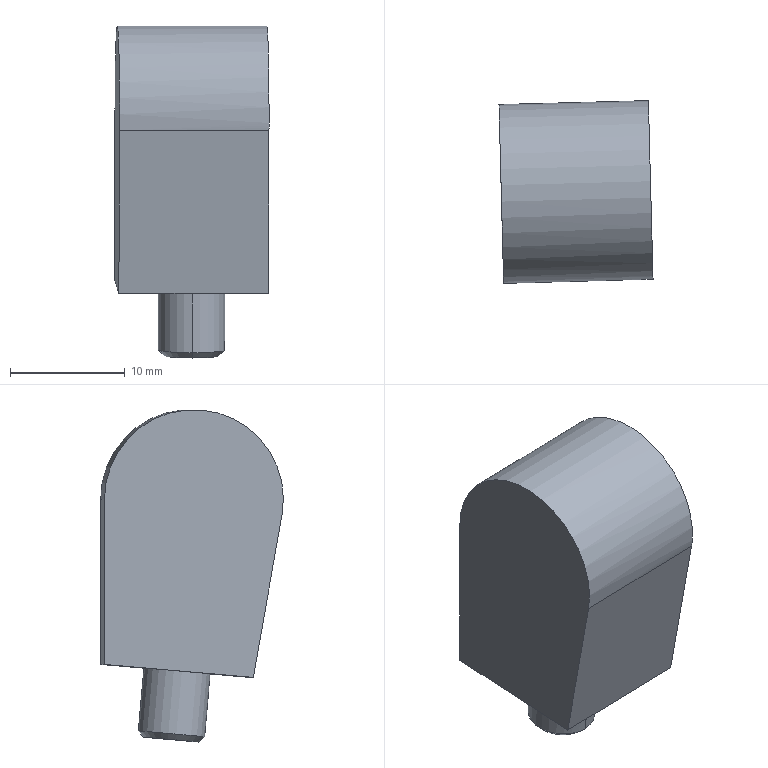Part | STEP file | 1_id1058_x_t | 1 solid | 11 faces | box 13.4 x 15.898 x 28.911 mm | volume 4184 mm3 | plane 6 | cylinder 3 | cone 2 | commonest cylinder face diameters 5.795 x2 15.565 x1
STEP:
#1=CARTESIAN_POINT('',(0.,0.,0.));
#2=DIRECTION('',(0.,0.,1.));
#3=DIRECTION('',(1.,0.,0.));
#4=AXIS2_PLACEMENT_3D('',#1,#2,#3);
#5=CARTESIAN_POINT('',(972.745,345.028,-29.863));
#6=VERTEX_POINT('',#5);
#7=CARTESIAN_POINT('',(972.733,345.49,-29.313));
#8=VERTEX_POINT('',#7);
#9=CARTESIAN_POINT('',(972.745,345.028,-29.863));
#10=DIRECTION('',(-0.01672,0.6426,0.766));
#11=VECTOR('',#10,1.);
#12=LINE('',#9,#11);
#13=CARTESIAN_POINT('',(972.807,342.627,-29.819));
#14=DIRECTION('',(0.002266,-0.08713,0.9962));
#15=DIRECTION('',(-0.02591,0.9959,0.08716));
#16=AXIS2_PLACEMENT_3D('',#13,#14,#15);
#17=CONICAL_SURFACE('',#16,2.644,0.7854);
#18=CARTESIAN_POINT('',(6.283,-0.254));
#19=DIRECTION('',(0.,1.));
#20=VECTOR('',#19,1.);
#21=LINE('',#18,#20);
#22=(GEOMETRIC_REPRESENTATION_CONTEXT(2)PARAMETRIC_REPRESENTATION_CONTEXT()REPRESENTATION_CONTEXT('',''));
#23=DEFINITIONAL_REPRESENTATION('',(#21),#22);
#24=PCURVE('',#17,#23);
#25=CARTESIAN_POINT('',(972.807,342.627,-29.819));
#26=DIRECTION('',(0.002266,-0.08713,0.9962));
#27=DIRECTION('',(-0.02591,0.9959,0.08716));
#28=AXIS2_PLACEMENT_3D('',#25,#26,#27);
#29=CONICAL_SURFACE('',#28,2.644,0.7854);
#30=CARTESIAN_POINT('',(0.,-0.254));
#31=DIRECTION('',(0.,1.));
#32=VECTOR('',#31,1.);
#33=LINE('',#30,#32);
#34=(GEOMETRIC_REPRESENTATION_CONTEXT(2)PARAMETRIC_REPRESENTATION_CONTEXT()REPRESENTATION_CONTEXT('',''));
#35=DEFINITIONAL_REPRESENTATION('',(#33),#34);
#36=PCURVE('',#29,#35);
#37=SURFACE_CURVE('',#12,(#24,#36),.PCURVE_S1.);
#38=EDGE_CURVE('',#6,#8,#37,.T.);
#39=ORIENTED_EDGE('',*,*,#38,.T.);
#40=CARTESIAN_POINT('',(972.883,339.719,-29.818));
#41=VERTEX_POINT('',#40);
#42=CARTESIAN_POINT('',(972.808,342.604,-29.565));
#43=DIRECTION('',(0.002266,-0.08713,0.9962));
#44=DIRECTION('',(0.02591,-0.9959,-0.08716));
#45=AXIS2_PLACEMENT_3D('',#42,#43,#44);
#46=CIRCLE('',#45,2.898);
#47=CARTESIAN_POINT('',(3.142,0.254));
#48=DIRECTION('',(1.,0.));
#49=VECTOR('',#48,1.);
#50=LINE('',#47,#49);
#51=(GEOMETRIC_REPRESENTATION_CONTEXT(2)PARAMETRIC_REPRESENTATION_CONTEXT()REPRESENTATION_CONTEXT('',''));
#52=DEFINITIONAL_REPRESENTATION('',(#50),#51);
#53=PCURVE('',#17,#52);
#54=CARTESIAN_POINT('',(972.82,342.126,-24.094));
#55=DIRECTION('',(-0.002266,0.08713,-0.9962));
#56=DIRECTION('',(-0.02591,0.9959,0.08716));
#57=AXIS2_PLACEMENT_3D('',#54,#55,#56);
#58=CYLINDRICAL_SURFACE('',#57,2.898);
#59=CARTESIAN_POINT('',(3.142,5.492));
#60=DIRECTION('',(-1.,0.));
#61=VECTOR('',#60,1.);
#62=LINE('',#59,#61);
#63=(GEOMETRIC_REPRESENTATION_CONTEXT(2)PARAMETRIC_REPRESENTATION_CONTEXT()REPRESENTATION_CONTEXT('',''));
#64=DEFINITIONAL_REPRESENTATION('',(#62),#63);
#65=PCURVE('',#58,#64);
#66=SURFACE_CURVE('',#46,(#53,#65),.PCURVE_S1.);
#67=EDGE_CURVE('',#41,#8,#66,.T.);
#68=ORIENTED_EDGE('',*,*,#67,.F.);
#69=CARTESIAN_POINT('',(972.869,340.269,-30.28));
#70=VERTEX_POINT('',#69);
#71=CARTESIAN_POINT('',(972.869,340.269,-30.28));
#72=DIRECTION('',(-0.01992,0.7658,-0.6428));
#73=VECTOR('',#72,1.);
#74=LINE('',#71,#73);
#75=CARTESIAN_POINT('',(3.142,-0.254));
#76=DIRECTION('',(0.,-1.));
#77=VECTOR('',#76,1.);
#78=LINE('',#75,#77);
#79=(GEOMETRIC_REPRESENTATION_CONTEXT(2)PARAMETRIC_REPRESENTATION_CONTEXT()REPRESENTATION_CONTEXT('',''));
#80=DEFINITIONAL_REPRESENTATION('',(#78),#79);
#81=PCURVE('',#17,#80);
#82=CARTESIAN_POINT('',(3.142,-0.254));
#83=DIRECTION('',(0.,-1.));
#84=VECTOR('',#83,1.);
#85=LINE('',#82,#84);
#86=(GEOMETRIC_REPRESENTATION_CONTEXT(2)PARAMETRIC_REPRESENTATION_CONTEXT()REPRESENTATION_CONTEXT('',''));
#87=DEFINITIONAL_REPRESENTATION('',(#85),#86);
#88=PCURVE('',#29,#87);
#89=SURFACE_CURVE('',#74,(#81,#88),.PCURVE_S1.);
#90=EDGE_CURVE('',#41,#70,#89,.T.);
#91=ORIENTED_EDGE('',*,*,#90,.T.);
#92=CARTESIAN_POINT('',(972.807,342.649,-30.072));
#93=DIRECTION('',(-0.002266,0.08713,-0.9962));
#94=DIRECTION('',(-0.02591,0.9959,0.08716));
#95=AXIS2_PLACEMENT_3D('',#92,#93,#94);
#96=CIRCLE('',#95,2.39);
#97=CARTESIAN_POINT('',(6.283,-0.254));
#98=DIRECTION('',(-1.,0.));
#99=VECTOR('',#98,1.);
#100=LINE('',#97,#99);
#101=(GEOMETRIC_REPRESENTATION_CONTEXT(2)PARAMETRIC_REPRESENTATION_CONTEXT()REPRESENTATION_CONTEXT('',''));
#102=DEFINITIONAL_REPRESENTATION('',(#100),#101);
#103=PCURVE('',#17,#102);
#104=CARTESIAN_POINT('',(972.807,342.649,-30.072));
#105=DIRECTION('',(-0.002266,0.08713,-0.9962));
#106=DIRECTION('',(0.8426,0.5366,0.04501));
#107=AXIS2_PLACEMENT_3D('',#104,#105,#106);
#108=PLANE('',#107);
#109=CARTESIAN_POINT('',(0.,0.));
#110=DIRECTION('',(0.5165,-0.8563));
#111=AXIS2_PLACEMENT_2D('',#109,#110);
#112=CIRCLE('',#111,2.39);
#113=(GEOMETRIC_REPRESENTATION_CONTEXT(2)PARAMETRIC_REPRESENTATION_CONTEXT()REPRESENTATION_CONTEXT('',''));
#114=DEFINITIONAL_REPRESENTATION('',(#112),#113);
#115=PCURVE('',#108,#114);
#116=SURFACE_CURVE('',#96,(#103,#115),.PCURVE_S1.);
#117=EDGE_CURVE('',#6,#70,#116,.T.);
#118=ORIENTED_EDGE('',*,*,#117,.F.);
#119=EDGE_LOOP('',(#39,#68,#91,#118));
#120=FACE_BOUND('',#119,.T.);
#121=ADVANCED_FACE('',(#120),#17,.T.);
#122=CARTESIAN_POINT('',(972.807,342.649,-30.072));
#123=DIRECTION('',(-0.002266,0.08713,-0.9962));
#124=DIRECTION('',(0.02591,-0.9959,-0.08716));
#125=AXIS2_PLACEMENT_3D('',#122,#123,#124);
#126=CIRCLE('',#125,2.39);
#127=CARTESIAN_POINT('',(0.,0.));
#128=DIRECTION('',(-0.5165,0.8563));
#129=AXIS2_PLACEMENT_2D('',#127,#128);
#130=CIRCLE('',#129,2.39);
#131=(GEOMETRIC_REPRESENTATION_CONTEXT(2)PARAMETRIC_REPRESENTATION_CONTEXT()REPRESENTATION_CONTEXT('',''));
#132=DEFINITIONAL_REPRESENTATION('',(#130),#131);
#133=PCURVE('',#108,#132);
#134=CARTESIAN_POINT('',(3.142,-0.254));
#135=DIRECTION('',(-1.,0.));
#136=VECTOR('',#135,1.);
#137=LINE('',#134,#136);
#138=(GEOMETRIC_REPRESENTATION_CONTEXT(2)PARAMETRIC_REPRESENTATION_CONTEXT()REPRESENTATION_CONTEXT('',''));
#139=DEFINITIONAL_REPRESENTATION('',(#137),#138);
#140=PCURVE('',#29,#139);
#141=SURFACE_CURVE('',#126,(#133,#140),.PCURVE_S1.);
#142=EDGE_CURVE('',#70,#6,#141,.T.);
#143=ORIENTED_EDGE('',*,*,#142,.T.);
#144=ORIENTED_EDGE('',*,*,#117,.T.);
#145=EDGE_LOOP('',(#143,#144));
#146=FACE_BOUND('',#145,.T.);
#147=ADVANCED_FACE('',(#146),#108,.T.);
#148=ORIENTED_EDGE('',*,*,#90,.F.);
#149=CARTESIAN_POINT('',(972.808,342.604,-29.565));
#150=DIRECTION('',(0.002266,-0.08713,0.9962));
#151=DIRECTION('',(-0.02591,0.9959,0.08716));
#152=AXIS2_PLACEMENT_3D('',#149,#150,#151);
#153=CIRCLE('',#152,2.898);
#154=CARTESIAN_POINT('',(0.,0.254));
#155=DIRECTION('',(1.,0.));
#156=VECTOR('',#155,1.);
#157=LINE('',#154,#156);
#158=(GEOMETRIC_REPRESENTATION_CONTEXT(2)PARAMETRIC_REPRESENTATION_CONTEXT()REPRESENTATION_CONTEXT('',''));
#159=DEFINITIONAL_REPRESENTATION('',(#157),#158);
#160=PCURVE('',#29,#159);
#161=CARTESIAN_POINT('',(972.82,342.126,-24.094));
#162=DIRECTION('',(-0.002266,0.08713,-0.9962));
#163=DIRECTION('',(-0.02591,0.9959,0.08716));
#164=AXIS2_PLACEMENT_3D('',#161,#162,#163);
#165=CYLINDRICAL_SURFACE('',#164,2.898);
#166=CARTESIAN_POINT('',(6.283,5.492));
#167=DIRECTION('',(-1.,0.));
#168=VECTOR('',#167,1.);
#169=LINE('',#166,#168);
#170=(GEOMETRIC_REPRESENTATION_CONTEXT(2)PARAMETRIC_REPRESENTATION_CONTEXT()REPRESENTATION_CONTEXT('',''));
#171=DEFINITIONAL_REPRESENTATION('',(#169),#170);
#172=PCURVE('',#165,#171);
#173=SURFACE_CURVE('',#153,(#160,#172),.PCURVE_S1.);
#174=EDGE_CURVE('',#8,#41,#173,.T.);
#175=ORIENTED_EDGE('',*,*,#174,.F.);
#176=ORIENTED_EDGE('',*,*,#38,.F.);
#177=ORIENTED_EDGE('',*,*,#142,.F.);
#178=EDGE_LOOP('',(#148,#175,#176,#177));
#179=FACE_BOUND('',#178,.T.);
#180=ADVANCED_FACE('',(#179),#29,.T.);
#181=CARTESIAN_POINT('',(972.895,339.24,-24.347));
#182=VERTEX_POINT('',#181);
#183=CARTESIAN_POINT('',(972.895,339.24,-24.347));
#184=DIRECTION('',(0.002266,-0.08713,0.9962));
#185=VECTOR('',#184,1.);
#186=LINE('',#183,#185);
#187=CARTESIAN_POINT('',(3.142,0.));
#188=DIRECTION('',(0.,-1.));
#189=VECTOR('',#188,1.);
#190=LINE('',#187,#189);
#191=(GEOMETRIC_REPRESENTATION_CONTEXT(2)PARAMETRIC_REPRESENTATION_CONTEXT()REPRESENTATION_CONTEXT('',''));
#192=DEFINITIONAL_REPRESENTATION('',(#190),#191);
#193=PCURVE('',#165,#192);
#194=CARTESIAN_POINT('',(3.142,0.));
#195=DIRECTION('',(0.,-1.));
#196=VECTOR('',#195,1.);
#197=LINE('',#194,#196);
#198=(GEOMETRIC_REPRESENTATION_CONTEXT(2)PARAMETRIC_REPRESENTATION_CONTEXT()REPRESENTATION_CONTEXT('',''));
#199=DEFINITIONAL_REPRESENTATION('',(#197),#198);
#200=PCURVE('',#58,#199);
#201=SURFACE_CURVE('',#186,(#193,#200),.PCURVE_S1.);
#202=EDGE_CURVE('',#41,#182,#201,.T.);
#203=ORIENTED_EDGE('',*,*,#202,.T.);
#204=CARTESIAN_POINT('',(972.745,345.011,-23.842));
#205=VERTEX_POINT('',#204);
#206=CARTESIAN_POINT('',(972.82,342.126,-24.094));
#207=DIRECTION('',(0.002266,-0.08713,0.9962));
#208=DIRECTION('',(-0.02591,0.9959,0.08716));
#209=AXIS2_PLACEMENT_3D('',#206,#207,#208);
#210=CIRCLE('',#209,2.898);
#211=CARTESIAN_POINT('',(6.283,0.));
#212=DIRECTION('',(-1.,0.));
#213=VECTOR('',#212,1.);
#214=LINE('',#211,#213);
#215=(GEOMETRIC_REPRESENTATION_CONTEXT(2)PARAMETRIC_REPRESENTATION_CONTEXT()REPRESENTATION_CONTEXT('',''));
#216=DEFINITIONAL_REPRESENTATION('',(#214),#215);
#217=PCURVE('',#165,#216);
#218=CARTESIAN_POINT('',(979.15,348.768,-23.528));
#219=DIRECTION('',(-0.002266,0.08713,-0.9962));
#220=DIRECTION('',(0.8426,0.5366,0.04501));
#221=AXIS2_PLACEMENT_3D('',#218,#219,#220);
#222=PLANE('',#221);
#223=CARTESIAN_POINT('',(-7.427,-0.2723));
#224=CARTESIAN_POINT('',(-11.724,-2.864));
#225=CARTESIAN_POINT('',(-11.82,2.153));
#226=CARTESIAN_POINT('',(-11.916,7.171));
#227=CARTESIAN_POINT('',(-7.523,4.745));
#228=CARTESIAN_POINT('',(-3.129,2.32));
#229=CARTESIAN_POINT('',(-7.427,-0.2723));
#230=(BOUNDED_CURVE()B_SPLINE_CURVE(2,(#223,#224,#225,#226,#227,#228,#229),.UNSPECIFIED.,.T.,.F.)B_SPLINE_CURVE_WITH_KNOTS((1,2,2,2,2,1),(-2.094,0.,2.094,4.189,6.283,8.378),.UNSPECIFIED.)CURVE()GEOMETRIC_REPRESENTATION_ITEM()RATIONAL_B_SPLINE_CURVE((1.,0.5,1.,0.5,1.,0.5,1.))REPRESENTATION_ITEM(''));
#231=(GEOMETRIC_REPRESENTATION_CONTEXT(2)PARAMETRIC_REPRESENTATION_CONTEXT()REPRESENTATION_CONTEXT('',''));
#232=DEFINITIONAL_REPRESENTATION('',(#230),#231);
#233=PCURVE('',#222,#232);
#234=SURFACE_CURVE('',#210,(#217,#233),.PCURVE_S1.);
#235=EDGE_CURVE('',#205,#182,#234,.T.);
#236=ORIENTED_EDGE('',*,*,#235,.F.);
#237=CARTESIAN_POINT('',(972.745,345.011,-23.842));
#238=DIRECTION('',(-0.002266,0.08713,-0.9962));
#239=VECTOR('',#238,1.);
#240=LINE('',#237,#239);
#241=CARTESIAN_POINT('',(6.283,0.));
#242=DIRECTION('',(0.,1.));
#243=VECTOR('',#242,1.);
#244=LINE('',#241,#243);
#245=(GEOMETRIC_REPRESENTATION_CONTEXT(2)PARAMETRIC_REPRESENTATION_CONTEXT()REPRESENTATION_CONTEXT('',''));
#246=DEFINITIONAL_REPRESENTATION('',(#244),#245);
#247=PCURVE('',#165,#246);
#248=CARTESIAN_POINT('',(0.,0.));
#249=DIRECTION('',(0.,1.));
#250=VECTOR('',#249,1.);
#251=LINE('',#248,#250);
#252=(GEOMETRIC_REPRESENTATION_CONTEXT(2)PARAMETRIC_REPRESENTATION_CONTEXT()REPRESENTATION_CONTEXT('',''));
#253=DEFINITIONAL_REPRESENTATION('',(#251),#252);
#254=PCURVE('',#58,#253);
#255=SURFACE_CURVE('',#240,(#247,#254),.PCURVE_S1.);
#256=EDGE_CURVE('',#205,#8,#255,.T.);
#257=ORIENTED_EDGE('',*,*,#256,.T.);
#258=ORIENTED_EDGE('',*,*,#174,.T.);
#259=EDGE_LOOP('',(#203,#236,#257,#258));
#260=FACE_BOUND('',#259,.T.);
#261=ADVANCED_FACE('',(#260),#165,.T.);
#262=ORIENTED_EDGE('',*,*,#256,.F.);
#263=CARTESIAN_POINT('',(972.82,342.126,-24.094));
#264=DIRECTION('',(0.002266,-0.08713,0.9962));
#265=DIRECTION('',(0.02591,-0.9959,-0.08716));
#266=AXIS2_PLACEMENT_3D('',#263,#264,#265);
#267=CIRCLE('',#266,2.898);
#268=CARTESIAN_POINT('',(3.142,0.));
#269=DIRECTION('',(-1.,0.));
#270=VECTOR('',#269,1.);
#271=LINE('',#268,#270);
#272=(GEOMETRIC_REPRESENTATION_CONTEXT(2)PARAMETRIC_REPRESENTATION_CONTEXT()REPRESENTATION_CONTEXT('',''));
#273=DEFINITIONAL_REPRESENTATION('',(#271),#272);
#274=PCURVE('',#58,#273);
#275=CARTESIAN_POINT('',(-10.42,4.69));
#276=CARTESIAN_POINT('',(-6.122,7.282));
#277=CARTESIAN_POINT('',(-6.026,2.264));
#278=CARTESIAN_POINT('',(-5.93,-2.753));
#279=CARTESIAN_POINT('',(-10.324,-0.3278));
#280=CARTESIAN_POINT('',(-14.717,2.098));
#281=CARTESIAN_POINT('',(-10.42,4.69));
#282=(BOUNDED_CURVE()B_SPLINE_CURVE(2,(#275,#276,#277,#278,#279,#280,#281),.UNSPECIFIED.,.T.,.F.)B_SPLINE_CURVE_WITH_KNOTS((1,2,2,2,2,1),(-2.094,0.,2.094,4.189,6.283,8.378),.UNSPECIFIED.)CURVE()GEOMETRIC_REPRESENTATION_ITEM()RATIONAL_B_SPLINE_CURVE((1.,0.5,1.,0.5,1.,0.5,1.))REPRESENTATION_ITEM(''));
#283=(GEOMETRIC_REPRESENTATION_CONTEXT(2)PARAMETRIC_REPRESENTATION_CONTEXT()REPRESENTATION_CONTEXT('',''));
#284=DEFINITIONAL_REPRESENTATION('',(#282),#283);
#285=PCURVE('',#222,#284);
#286=SURFACE_CURVE('',#267,(#274,#285),.PCURVE_S1.);
#287=EDGE_CURVE('',#182,#205,#286,.T.);
#288=ORIENTED_EDGE('',*,*,#287,.F.);
#289=ORIENTED_EDGE('',*,*,#202,.F.);
#290=ORIENTED_EDGE('',*,*,#67,.T.);
#291=EDGE_LOOP('',(#262,#288,#289,#290));
#292=FACE_BOUND('',#291,.T.);
#293=ADVANCED_FACE('',(#292),#58,.T.);
#294=CARTESIAN_POINT('',(966.154,348.43,-23.528));
#295=VERTEX_POINT('',#294);
#296=CARTESIAN_POINT('',(979.15,348.768,-23.528));
#297=VERTEX_POINT('',#296);
#298=CARTESIAN_POINT('',(966.154,348.43,-23.528));
#299=DIRECTION('',(0.9997,0.02601,0.));
#300=VECTOR('',#299,1.);
#301=LINE('',#298,#300);
#302=CARTESIAN_POINT('',(-11.132,-6.714));
#303=DIRECTION('',(0.8563,0.5165));
#304=VECTOR('',#303,1.);
#305=LINE('',#302,#304);
#306=(GEOMETRIC_REPRESENTATION_CONTEXT(2)PARAMETRIC_REPRESENTATION_CONTEXT()REPRESENTATION_CONTEXT('',''));
#307=DEFINITIONAL_REPRESENTATION('',(#305),#306);
#308=PCURVE('',#222,#307);
#309=CARTESIAN_POINT('',(979.15,348.768,-9.151));
#310=DIRECTION('',(-0.02601,0.9997,0.));
#311=DIRECTION('',(0.,0.,-1.));
#312=AXIS2_PLACEMENT_3D('',#309,#310,#311);
#313=PLANE('',#312);
#314=CARTESIAN_POINT('',(14.376,13.));
#315=DIRECTION('',(0.,-1.));
#316=VECTOR('',#315,1.);
#317=LINE('',#314,#316);
#318=(GEOMETRIC_REPRESENTATION_CONTEXT(2)PARAMETRIC_REPRESENTATION_CONTEXT()REPRESENTATION_CONTEXT('',''));
#319=DEFINITIONAL_REPRESENTATION('',(#317),#318);
#320=PCURVE('',#313,#319);
#321=SURFACE_CURVE('',#301,(#308,#320),.PCURVE_S1.);
#322=EDGE_CURVE('',#295,#297,#321,.T.);
#323=ORIENTED_EDGE('',*,*,#322,.T.);
#324=CARTESIAN_POINT('',(979.487,335.822,-24.661));
#325=VERTEX_POINT('',#324);
#326=CARTESIAN_POINT('',(979.487,335.822,-24.661));
#327=DIRECTION('',(-0.02591,0.9959,0.08716));
#328=VECTOR('',#327,1.);
#329=LINE('',#326,#328);
#330=CARTESIAN_POINT('',(-6.714,11.132));
#331=DIRECTION('',(0.5165,-0.8563));
#332=VECTOR('',#331,1.);
#333=LINE('',#330,#332);
#334=(GEOMETRIC_REPRESENTATION_CONTEXT(2)PARAMETRIC_REPRESENTATION_CONTEXT()REPRESENTATION_CONTEXT('',''));
#335=DEFINITIONAL_REPRESENTATION('',(#333),#334);
#336=PCURVE('',#222,#335);
#337=CARTESIAN_POINT('',(979.352,340.988,-9.151));
#338=DIRECTION('',(0.9997,0.02601,0.));
#339=DIRECTION('',(0.02601,-0.9997,0.));
#340=AXIS2_PLACEMENT_3D('',#337,#338,#339);
#341=PLANE('',#340);
#342=CARTESIAN_POINT('',(5.168,15.509));
#343=DIRECTION('',(-0.9962,-0.08716));
#344=VECTOR('',#343,1.);
#345=LINE('',#342,#344);
#346=(GEOMETRIC_REPRESENTATION_CONTEXT(2)PARAMETRIC_REPRESENTATION_CONTEXT()REPRESENTATION_CONTEXT('',''));
#347=DEFINITIONAL_REPRESENTATION('',(#345),#346);
#348=PCURVE('',#341,#347);
#349=SURFACE_CURVE('',#329,(#336,#348),.PCURVE_S1.);
#350=EDGE_CURVE('',#325,#297,#349,.T.);
#351=ORIENTED_EDGE('',*,*,#350,.F.);
#352=CARTESIAN_POINT('',(966.491,335.484,-24.661));
#353=VERTEX_POINT('',#352);
#354=CARTESIAN_POINT('',(966.491,335.484,-24.661));
#355=DIRECTION('',(0.9997,0.02601,0.));
#356=VECTOR('',#355,1.);
#357=LINE('',#354,#356);
#358=CARTESIAN_POINT('',(-17.846,4.418));
#359=DIRECTION('',(0.8563,0.5165));
#360=VECTOR('',#359,1.);
#361=LINE('',#358,#360);
#362=(GEOMETRIC_REPRESENTATION_CONTEXT(2)PARAMETRIC_REPRESENTATION_CONTEXT()REPRESENTATION_CONTEXT('',''));
#363=DEFINITIONAL_REPRESENTATION('',(#361),#362);
#364=PCURVE('',#222,#363);
#365=CARTESIAN_POINT('',(979.551,333.326,-10.503));
#366=DIRECTION('',(-0.02561,0.9845,0.1736));
#367=DIRECTION('',(0.2732,0.174,-0.9461));
#368=AXIS2_PLACEMENT_3D('',#365,#366,#367);
#369=PLANE('',#368);
#370=CARTESIAN_POINT('',(10.202,16.48));
#371=DIRECTION('',(0.2776,-0.9607));
#372=VECTOR('',#371,1.);
#373=LINE('',#370,#372);
#374=(GEOMETRIC_REPRESENTATION_CONTEXT(2)PARAMETRIC_REPRESENTATION_CONTEXT()REPRESENTATION_CONTEXT('',''));
#375=DEFINITIONAL_REPRESENTATION('',(#373),#374);
#376=PCURVE('',#369,#375);
#377=SURFACE_CURVE('',#357,(#364,#376),.PCURVE_S1.);
#378=EDGE_CURVE('',#353,#325,#377,.T.);
#379=ORIENTED_EDGE('',*,*,#378,.F.);
#380=CARTESIAN_POINT('',(966.491,335.484,-24.661));
#381=DIRECTION('',(-0.02591,0.9959,0.08716));
#382=VECTOR('',#381,1.);
#383=LINE('',#380,#382);
#384=CARTESIAN_POINT('',(-17.846,4.418));
#385=DIRECTION('',(0.5165,-0.8563));
#386=VECTOR('',#385,1.);
#387=LINE('',#384,#386);
#388=(GEOMETRIC_REPRESENTATION_CONTEXT(2)PARAMETRIC_REPRESENTATION_CONTEXT()REPRESENTATION_CONTEXT('',''));
#389=DEFINITIONAL_REPRESENTATION('',(#387),#388);
#390=PCURVE('',#222,#389);
#391=CARTESIAN_POINT('',(966.357,340.65,-9.151));
#392=DIRECTION('',(0.9997,0.02601,0.));
#393=DIRECTION('',(0.02601,-0.9997,0.));
#394=AXIS2_PLACEMENT_3D('',#391,#392,#393);
#395=PLANE('',#394);
#396=CARTESIAN_POINT('',(5.168,15.509));
#397=DIRECTION('',(-0.9962,-0.08716));
#398=VECTOR('',#397,1.);
#399=LINE('',#396,#398);
#400=(GEOMETRIC_REPRESENTATION_CONTEXT(2)PARAMETRIC_REPRESENTATION_CONTEXT()REPRESENTATION_CONTEXT('',''));
#401=DEFINITIONAL_REPRESENTATION('',(#399),#400);
#402=PCURVE('',#395,#401);
#403=SURFACE_CURVE('',#383,(#390,#402),.PCURVE_S1.);
#404=EDGE_CURVE('',#353,#295,#403,.T.);
#405=ORIENTED_EDGE('',*,*,#404,.T.);
#406=EDGE_LOOP('',(#323,#351,#379,#405));
#407=FACE_BOUND('',#406,.T.);
#408=ORIENTED_EDGE('',*,*,#287,.T.);
#409=ORIENTED_EDGE('',*,*,#235,.T.);
#410=EDGE_LOOP('',(#408,#409));
#411=FACE_BOUND('',#410,.T.);
#412=ADVANCED_FACE('',(#407,#411),#222,.T.);
#413=CARTESIAN_POINT('',(966.556,332.988,-10.503));
#414=VERTEX_POINT('',#413);
#415=CARTESIAN_POINT('',(966.491,335.484,-24.661));
#416=DIRECTION('',(0.004516,-0.1736,0.9848));
#417=VECTOR('',#416,1.);
#418=LINE('',#415,#417);
#419=CARTESIAN_POINT('',(5.168,15.509));
#420=DIRECTION('',(0.1736,-0.9848));
#421=VECTOR('',#420,1.);
#422=LINE('',#419,#421);
#423=(GEOMETRIC_REPRESENTATION_CONTEXT(2)PARAMETRIC_REPRESENTATION_CONTEXT()REPRESENTATION_CONTEXT('',''));
#424=DEFINITIONAL_REPRESENTATION('',(#422),#423);
#425=PCURVE('',#395,#424);
#426=CARTESIAN_POINT('',(10.202,16.48));
#427=DIRECTION('',(-0.9607,-0.2776));
#428=VECTOR('',#427,1.);
#429=LINE('',#426,#428);
#430=(GEOMETRIC_REPRESENTATION_CONTEXT(2)PARAMETRIC_REPRESENTATION_CONTEXT()REPRESENTATION_CONTEXT('',''));
#431=DEFINITIONAL_REPRESENTATION('',(#429),#430);
#432=PCURVE('',#369,#431);
#433=SURFACE_CURVE('',#418,(#425,#432),.PCURVE_S1.);
#434=EDGE_CURVE('',#353,#414,#433,.T.);
#435=ORIENTED_EDGE('',*,*,#434,.T.);
#436=CARTESIAN_POINT('',(966.374,339.972,-1.398));
#437=VERTEX_POINT('',#436);
#438=CARTESIAN_POINT('',(966.357,340.65,-9.151));
#439=DIRECTION('',(-0.9997,-0.02601,0.));
#440=DIRECTION('',(0.02561,-0.9845,-0.1736));
#441=AXIS2_PLACEMENT_3D('',#438,#439,#440);
#442=CIRCLE('',#441,7.783);
#443=CARTESIAN_POINT('',(7.664,1.351));
#444=CARTESIAN_POINT('',(10.005,-11.924));
#445=CARTESIAN_POINT('',(-2.662,-7.313));
#446=CARTESIAN_POINT('',(-15.329,-2.703));
#447=CARTESIAN_POINT('',(-5.003,5.962));
#448=CARTESIAN_POINT('',(5.324,14.627));
#449=CARTESIAN_POINT('',(7.664,1.351));
#450=(BOUNDED_CURVE()B_SPLINE_CURVE(2,(#443,#444,#445,#446,#447,#448,#449),.UNSPECIFIED.,.T.,.F.)B_SPLINE_CURVE_WITH_KNOTS((1,2,2,2,2,1),(-2.094,0.,2.094,4.189,6.283,8.378),.UNSPECIFIED.)CURVE()GEOMETRIC_REPRESENTATION_ITEM()RATIONAL_B_SPLINE_CURVE((1.,0.5,1.,0.5,1.,0.5,1.))REPRESENTATION_ITEM(''));
#451=(GEOMETRIC_REPRESENTATION_CONTEXT(2)PARAMETRIC_REPRESENTATION_CONTEXT()REPRESENTATION_CONTEXT('',''));
#452=DEFINITIONAL_REPRESENTATION('',(#450),#451);
#453=PCURVE('',#395,#452);
#454=CARTESIAN_POINT('',(979.352,340.988,-9.151));
#455=DIRECTION('',(-0.9997,-0.02601,0.));
#456=DIRECTION('',(-0.002266,0.08713,-0.9962));
#457=AXIS2_PLACEMENT_3D('',#454,#455,#456);
#458=CYLINDRICAL_SURFACE('',#457,7.783);
#459=CARTESIAN_POINT('',(1.484,13.));
#460=DIRECTION('',(1.,0.));
#461=VECTOR('',#460,1.);
#462=LINE('',#459,#461);
#463=(GEOMETRIC_REPRESENTATION_CONTEXT(2)PARAMETRIC_REPRESENTATION_CONTEXT()REPRESENTATION_CONTEXT('',''));
#464=DEFINITIONAL_REPRESENTATION('',(#462),#463);
#465=PCURVE('',#458,#464);
#466=SURFACE_CURVE('',#442,(#453,#465),.PCURVE_S1.);
#467=EDGE_CURVE('',#414,#437,#466,.T.);
#468=ORIENTED_EDGE('',*,*,#467,.T.);
#469=CARTESIAN_POINT('',(966.154,348.43,-9.151));
#470=VERTEX_POINT('',#469);
#471=CARTESIAN_POINT('',(966.357,340.65,-9.151));
#472=DIRECTION('',(-0.9997,-0.02601,0.));
#473=DIRECTION('',(0.002266,-0.08713,0.9962));
#474=AXIS2_PLACEMENT_3D('',#471,#472,#473);
#475=CIRCLE('',#474,7.783);
#476=CARTESIAN_POINT('',(0.6783,-7.753));
#477=CARTESIAN_POINT('',(-12.75,-8.928));
#478=CARTESIAN_POINT('',(-7.053,3.289));
#479=CARTESIAN_POINT('',(-1.357,15.506));
#480=CARTESIAN_POINT('',(6.375,4.464));
#481=CARTESIAN_POINT('',(14.107,-6.578));
#482=CARTESIAN_POINT('',(0.6783,-7.753));
#483=(BOUNDED_CURVE()B_SPLINE_CURVE(2,(#476,#477,#478,#479,#480,#481,#482),.UNSPECIFIED.,.T.,.F.)B_SPLINE_CURVE_WITH_KNOTS((1,2,2,2,2,1),(-2.094,0.,2.094,4.189,6.283,8.378),.UNSPECIFIED.)CURVE()GEOMETRIC_REPRESENTATION_ITEM()RATIONAL_B_SPLINE_CURVE((1.,0.5,1.,0.5,1.,0.5,1.))REPRESENTATION_ITEM(''));
#484=(GEOMETRIC_REPRESENTATION_CONTEXT(2)PARAMETRIC_REPRESENTATION_CONTEXT()REPRESENTATION_CONTEXT('',''));
#485=DEFINITIONAL_REPRESENTATION('',(#483),#484);
#486=PCURVE('',#395,#485);
#487=CARTESIAN_POINT('',(3.142,13.));
#488=DIRECTION('',(1.,0.));
#489=VECTOR('',#488,1.);
#490=LINE('',#487,#489);
#491=(GEOMETRIC_REPRESENTATION_CONTEXT(2)PARAMETRIC_REPRESENTATION_CONTEXT()REPRESENTATION_CONTEXT('',''));
#492=DEFINITIONAL_REPRESENTATION('',(#490),#491);
#493=PCURVE('',#458,#492);
#494=SURFACE_CURVE('',#475,(#486,#493),.PCURVE_S1.);
#495=EDGE_CURVE('',#437,#470,#494,.T.);
#496=ORIENTED_EDGE('',*,*,#495,.T.);
#497=CARTESIAN_POINT('',(966.154,348.43,-23.528));
#498=DIRECTION('',(0.,0.,1.));
#499=VECTOR('',#498,1.);
#500=LINE('',#497,#499);
#501=CARTESIAN_POINT('',(-7.783,14.376));
#502=DIRECTION('',(0.,-1.));
#503=VECTOR('',#502,1.);
#504=LINE('',#501,#503);
#505=(GEOMETRIC_REPRESENTATION_CONTEXT(2)PARAMETRIC_REPRESENTATION_CONTEXT()REPRESENTATION_CONTEXT('',''));
#506=DEFINITIONAL_REPRESENTATION('',(#504),#505);
#507=PCURVE('',#395,#506);
#508=CARTESIAN_POINT('',(14.376,13.));
#509=DIRECTION('',(-1.,0.));
#510=VECTOR('',#509,1.);
#511=LINE('',#508,#510);
#512=(GEOMETRIC_REPRESENTATION_CONTEXT(2)PARAMETRIC_REPRESENTATION_CONTEXT()REPRESENTATION_CONTEXT('',''));
#513=DEFINITIONAL_REPRESENTATION('',(#511),#512);
#514=PCURVE('',#313,#513);
#515=SURFACE_CURVE('',#500,(#507,#514),.PCURVE_S1.);
#516=EDGE_CURVE('',#295,#470,#515,.T.);
#517=ORIENTED_EDGE('',*,*,#516,.F.);
#518=ORIENTED_EDGE('',*,*,#404,.F.);
#519=EDGE_LOOP('',(#435,#468,#496,#517,#518));
#520=FACE_BOUND('',#519,.T.);
#521=ADVANCED_FACE('',(#520),#395,.F.);
#522=CARTESIAN_POINT('',(979.15,348.768,-9.151));
#523=VERTEX_POINT('',#522);
#524=CARTESIAN_POINT('',(979.15,348.768,-9.151));
#525=DIRECTION('',(-0.9997,-0.02601,0.));
#526=VECTOR('',#525,1.);
#527=LINE('',#524,#526);
#528=CARTESIAN_POINT('',(0.,0.));
#529=DIRECTION('',(0.,1.));
#530=VECTOR('',#529,1.);
#531=LINE('',#528,#530);
#532=(GEOMETRIC_REPRESENTATION_CONTEXT(2)PARAMETRIC_REPRESENTATION_CONTEXT()REPRESENTATION_CONTEXT('',''));
#533=DEFINITIONAL_REPRESENTATION('',(#531),#532);
#534=PCURVE('',#313,#533);
#535=CARTESIAN_POINT('',(4.8,0.));
#536=DIRECTION('',(0.,1.));
#537=VECTOR('',#536,1.);
#538=LINE('',#535,#537);
#539=(GEOMETRIC_REPRESENTATION_CONTEXT(2)PARAMETRIC_REPRESENTATION_CONTEXT()REPRESENTATION_CONTEXT('',''));
#540=DEFINITIONAL_REPRESENTATION('',(#538),#539);
#541=PCURVE('',#458,#540);
#542=SURFACE_CURVE('',#527,(#534,#541),.PCURVE_S1.);
#543=EDGE_CURVE('',#523,#470,#542,.T.);
#544=ORIENTED_EDGE('',*,*,#543,.F.);
#545=CARTESIAN_POINT('',(979.15,348.768,-23.528));
#546=DIRECTION('',(0.,0.,1.));
#547=VECTOR('',#546,1.);
#548=LINE('',#545,#547);
#549=CARTESIAN_POINT('',(14.376,0.));
#550=DIRECTION('',(-1.,0.));
#551=VECTOR('',#550,1.);
#552=LINE('',#549,#551);
#553=(GEOMETRIC_REPRESENTATION_CONTEXT(2)PARAMETRIC_REPRESENTATION_CONTEXT()REPRESENTATION_CONTEXT('',''));
#554=DEFINITIONAL_REPRESENTATION('',(#552),#553);
#555=PCURVE('',#313,#554);
#556=CARTESIAN_POINT('',(-7.783,14.376));
#557=DIRECTION('',(0.,-1.));
#558=VECTOR('',#557,1.);
#559=LINE('',#556,#558);
#560=(GEOMETRIC_REPRESENTATION_CONTEXT(2)PARAMETRIC_REPRESENTATION_CONTEXT()REPRESENTATION_CONTEXT('',''));
#561=DEFINITIONAL_REPRESENTATION('',(#559),#560);
#562=PCURVE('',#341,#561);
#563=SURFACE_CURVE('',#548,(#555,#562),.PCURVE_S1.);
#564=EDGE_CURVE('',#297,#523,#563,.T.);
#565=ORIENTED_EDGE('',*,*,#564,.F.);
#566=ORIENTED_EDGE('',*,*,#322,.F.);
#567=ORIENTED_EDGE('',*,*,#516,.T.);
#568=EDGE_LOOP('',(#544,#565,#566,#567));
#569=FACE_BOUND('',#568,.T.);
#570=ADVANCED_FACE('',(#569),#313,.T.);
#571=ORIENTED_EDGE('',*,*,#564,.T.);
#572=CARTESIAN_POINT('',(979.37,340.31,-1.398));
#573=VERTEX_POINT('',#572);
#574=CARTESIAN_POINT('',(979.352,340.988,-9.151));
#575=DIRECTION('',(0.9997,0.02601,0.));
#576=DIRECTION('',(-0.02601,0.9997,0.));
#577=AXIS2_PLACEMENT_3D('',#574,#575,#576);
#578=CIRCLE('',#577,7.783);
#579=CARTESIAN_POINT('',(0.,0.));
#580=DIRECTION('',(-1.,0.));
#581=AXIS2_PLACEMENT_2D('',#579,#580);
#582=CIRCLE('',#581,7.783);
#583=(GEOMETRIC_REPRESENTATION_CONTEXT(2)PARAMETRIC_REPRESENTATION_CONTEXT()REPRESENTATION_CONTEXT('',''));
#584=DEFINITIONAL_REPRESENTATION('',(#582),#583);
#585=PCURVE('',#341,#584);
#586=CARTESIAN_POINT('',(4.8,0.));
#587=DIRECTION('',(-1.,0.));
#588=VECTOR('',#587,1.);
#589=LINE('',#586,#588);
#590=(GEOMETRIC_REPRESENTATION_CONTEXT(2)PARAMETRIC_REPRESENTATION_CONTEXT()REPRESENTATION_CONTEXT('',''));
#591=DEFINITIONAL_REPRESENTATION('',(#589),#590);
#592=PCURVE('',#458,#591);
#593=SURFACE_CURVE('',#578,(#585,#592),.PCURVE_S1.);
#594=EDGE_CURVE('',#523,#573,#593,.T.);
#595=ORIENTED_EDGE('',*,*,#594,.T.);
#596=CARTESIAN_POINT('',(979.554,333.238,-9.83));
#597=VERTEX_POINT('',#596);
#598=CARTESIAN_POINT('',(979.352,340.988,-9.151));
#599=DIRECTION('',(0.9997,0.02601,0.));
#600=DIRECTION('',(0.002266,-0.08713,0.9962));
#601=AXIS2_PLACEMENT_3D('',#598,#599,#600);
#602=CIRCLE('',#601,7.783);
#603=CARTESIAN_POINT('',(0.,0.));
#604=DIRECTION('',(0.08716,-0.9962));
#605=AXIS2_PLACEMENT_2D('',#603,#604);
#606=CIRCLE('',#605,7.783);
#607=(GEOMETRIC_REPRESENTATION_CONTEXT(2)PARAMETRIC_REPRESENTATION_CONTEXT()REPRESENTATION_CONTEXT('',''));
#608=DEFINITIONAL_REPRESENTATION('',(#606),#607);
#609=PCURVE('',#341,#608);
#610=CARTESIAN_POINT('',(3.142,0.));
#611=DIRECTION('',(-1.,0.));
#612=VECTOR('',#611,1.);
#613=LINE('',#610,#612);
#614=(GEOMETRIC_REPRESENTATION_CONTEXT(2)PARAMETRIC_REPRESENTATION_CONTEXT()REPRESENTATION_CONTEXT('',''));
#615=DEFINITIONAL_REPRESENTATION('',(#613),#614);
#616=PCURVE('',#458,#615);
#617=SURFACE_CURVE('',#602,(#609,#616),.PCURVE_S1.);
#618=EDGE_CURVE('',#573,#597,#617,.T.);
#619=ORIENTED_EDGE('',*,*,#618,.T.);
#620=CARTESIAN_POINT('',(979.551,333.326,-10.503));
#621=VERTEX_POINT('',#620);
#622=CARTESIAN_POINT('',(979.352,340.988,-9.151));
#623=DIRECTION('',(0.9997,0.02601,0.));
#624=DIRECTION('',(0.02591,-0.9959,-0.08716));
#625=AXIS2_PLACEMENT_3D('',#622,#623,#624);
#626=CIRCLE('',#625,7.783);
#627=CARTESIAN_POINT('',(0.,0.));
#628=DIRECTION('',(0.9962,0.08716));
#629=AXIS2_PLACEMENT_2D('',#627,#628);
#630=CIRCLE('',#629,7.783);
#631=(GEOMETRIC_REPRESENTATION_CONTEXT(2)PARAMETRIC_REPRESENTATION_CONTEXT()REPRESENTATION_CONTEXT('',''));
#632=DEFINITIONAL_REPRESENTATION('',(#630),#631);
#633=PCURVE('',#341,#632);
#634=CARTESIAN_POINT('',(1.571,0.));
#635=DIRECTION('',(-1.,0.));
#636=VECTOR('',#635,1.);
#637=LINE('',#634,#636);
#638=(GEOMETRIC_REPRESENTATION_CONTEXT(2)PARAMETRIC_REPRESENTATION_CONTEXT()REPRESENTATION_CONTEXT('',''));
#639=DEFINITIONAL_REPRESENTATION('',(#637),#638);
#640=PCURVE('',#458,#639);
#641=SURFACE_CURVE('',#626,(#633,#640),.PCURVE_S1.);
#642=EDGE_CURVE('',#597,#621,#641,.T.);
#643=ORIENTED_EDGE('',*,*,#642,.T.);
#644=CARTESIAN_POINT('',(979.487,335.822,-24.661));
#645=DIRECTION('',(0.004516,-0.1736,0.9848));
#646=VECTOR('',#645,1.);
#647=LINE('',#644,#646);
#648=CARTESIAN_POINT('',(5.168,15.509));
#649=DIRECTION('',(0.1736,-0.9848));
#650=VECTOR('',#649,1.);
#651=LINE('',#648,#650);
#652=(GEOMETRIC_REPRESENTATION_CONTEXT(2)PARAMETRIC_REPRESENTATION_CONTEXT()REPRESENTATION_CONTEXT('',''));
#653=DEFINITIONAL_REPRESENTATION('',(#651),#652);
#654=PCURVE('',#341,#653);
#655=CARTESIAN_POINT('',(13.811,3.991));
#656=DIRECTION('',(-0.9607,-0.2776));
#657=VECTOR('',#656,1.);
#658=LINE('',#655,#657);
#659=(GEOMETRIC_REPRESENTATION_CONTEXT(2)PARAMETRIC_REPRESENTATION_CONTEXT()REPRESENTATION_CONTEXT('',''));
#660=DEFINITIONAL_REPRESENTATION('',(#658),#659);
#661=PCURVE('',#369,#660);
#662=SURFACE_CURVE('',#647,(#654,#661),.PCURVE_S1.);
#663=EDGE_CURVE('',#325,#621,#662,.T.);
#664=ORIENTED_EDGE('',*,*,#663,.F.);
#665=ORIENTED_EDGE('',*,*,#350,.T.);
#666=EDGE_LOOP('',(#571,#595,#619,#643,#664,#665));
#667=FACE_BOUND('',#666,.T.);
#668=ADVANCED_FACE('',(#667),#341,.T.);
#669=ORIENTED_EDGE('',*,*,#378,.T.);
#670=ORIENTED_EDGE('',*,*,#663,.T.);
#671=CARTESIAN_POINT('',(979.551,333.326,-10.503));
#672=DIRECTION('',(-0.9997,-0.02601,0.));
#673=VECTOR('',#672,1.);
#674=LINE('',#671,#673);
#675=CARTESIAN_POINT('',(0.,0.));
#676=DIRECTION('',(-0.2776,0.9607));
#677=VECTOR('',#676,1.);
#678=LINE('',#675,#677);
#679=(GEOMETRIC_REPRESENTATION_CONTEXT(2)PARAMETRIC_REPRESENTATION_CONTEXT()REPRESENTATION_CONTEXT('',''));
#680=DEFINITIONAL_REPRESENTATION('',(#678),#679);
#681=PCURVE('',#369,#680);
#682=CARTESIAN_POINT('',(1.484,0.));
#683=DIRECTION('',(0.,1.));
#684=VECTOR('',#683,1.);
#685=LINE('',#682,#684);
#686=(GEOMETRIC_REPRESENTATION_CONTEXT(2)PARAMETRIC_REPRESENTATION_CONTEXT()REPRESENTATION_CONTEXT('',''));
#687=DEFINITIONAL_REPRESENTATION('',(#685),#686);
#688=PCURVE('',#458,#687);
#689=SURFACE_CURVE('',#674,(#681,#688),.PCURVE_S1.);
#690=EDGE_CURVE('',#621,#414,#689,.T.);
#691=ORIENTED_EDGE('',*,*,#690,.T.);
#692=ORIENTED_EDGE('',*,*,#434,.F.);
#693=EDGE_LOOP('',(#669,#670,#691,#692));
#694=FACE_BOUND('',#693,.T.);
#695=ADVANCED_FACE('',(#694),#369,.F.);
#696=ORIENTED_EDGE('',*,*,#467,.F.);
#697=ORIENTED_EDGE('',*,*,#690,.F.);
#698=ORIENTED_EDGE('',*,*,#642,.F.);
#699=ORIENTED_EDGE('',*,*,#618,.F.);
#700=ORIENTED_EDGE('',*,*,#594,.F.);
#701=ORIENTED_EDGE('',*,*,#543,.T.);
#702=ORIENTED_EDGE('',*,*,#495,.F.);
#703=EDGE_LOOP('',(#696,#697,#698,#699,#700,#701,#702));
#704=FACE_BOUND('',#703,.T.);
#705=ADVANCED_FACE('',(#704),#458,.T.);
#706=CLOSED_SHELL('',(#121,#147,#180,#261,#293,#412,#521,#570,#668,#695,#705));
#707=MANIFOLD_SOLID_BREP('',#706);
#708=(LENGTH_UNIT()NAMED_UNIT(*)SI_UNIT(.MILLI.,.METRE.));
#709=UNCERTAINTY_MEASURE_WITH_UNIT(LENGTH_MEASURE(0.0000001),#708,'','');
#710=(NAMED_UNIT(*)PLANE_ANGLE_UNIT()SI_UNIT($,.RADIAN.));
#711=(NAMED_UNIT(*)SI_UNIT($,.STERADIAN.)SOLID_ANGLE_UNIT());
#712=(GEOMETRIC_REPRESENTATION_CONTEXT(3)GLOBAL_UNCERTAINTY_ASSIGNED_CONTEXT((#709))GLOBAL_UNIT_ASSIGNED_CONTEXT((#708,#710,#711))REPRESENTATION_CONTEXT('',''));
#713=ADVANCED_BREP_SHAPE_REPRESENTATION('',(#4,#707),#712);